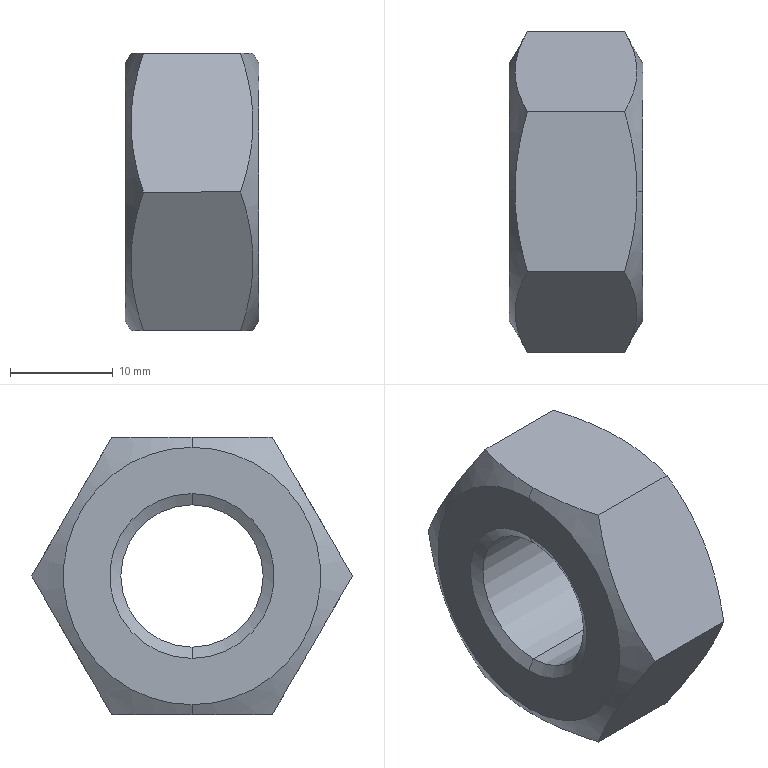Part | STEP file | DIN 6915 M16 | 1 solid | 18 faces | box 13 x 31.177 x 27 mm | volume 6064 mm3 | cone 8 | plane 8 | cylinder 2 | commonest cylinder face diameters 13.835 x2